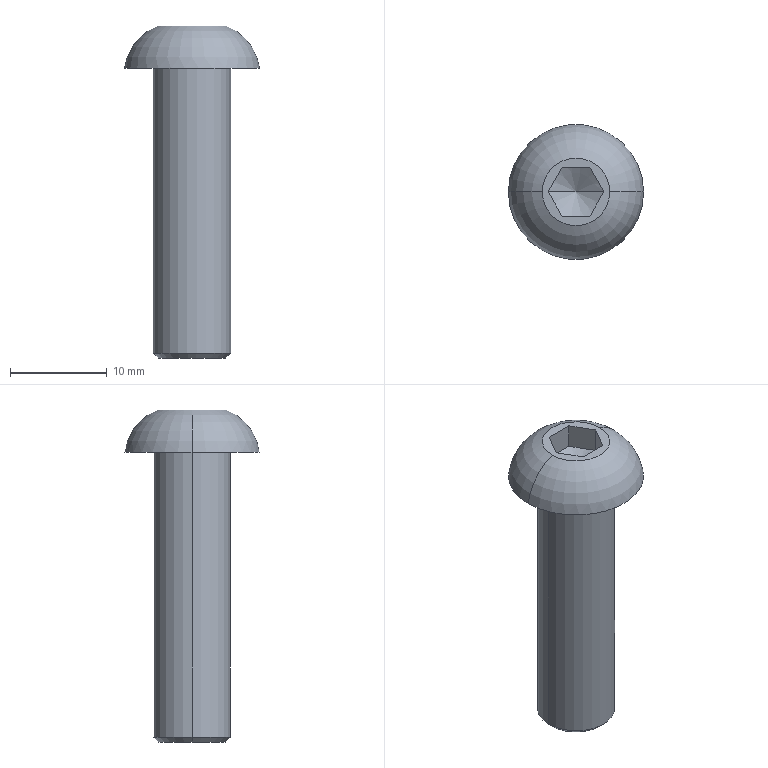Part | NX | features BREP 1 | 1 solid | 18 faces | box 14 x 14 x 34.4 mm | volume 1931 mm3 | plane 10 | cone 4 | torus 2 | cylinder 2 | commonest cylinder face diameters 8 x2
STEP:
#1=CARTESIAN_POINT('',(0.,0.,0.06795));
#2=VERTEX_POINT('',#1);
#3=CARTESIAN_POINT('',(-3.,0.,1.8));
#4=VERTEX_POINT('',#3);
#5=CARTESIAN_POINT('',(-3.,0.,1.8));
#6=DIRECTION('',(-0.866,0.,0.5));
#7=VECTOR('',#6,1000.);
#8=LINE('',#5,#7);
#9=EDGE_CURVE('',#2,#4,#8,.T.);
#10=ORIENTED_EDGE('',*,*,#9,.F.);
#11=CARTESIAN_POINT('',(3.,0.,1.8));
#12=VERTEX_POINT('',#11);
#13=CARTESIAN_POINT('',(3.,0.,1.8));
#14=DIRECTION('',(0.866,0.,0.5));
#15=VECTOR('',#14,1000.);
#16=LINE('',#13,#15);
#17=EDGE_CURVE('',#2,#12,#16,.T.);
#18=ORIENTED_EDGE('',*,*,#17,.T.);
#19=CARTESIAN_POINT('',(0.,0.,1.8));
#20=DIRECTION('',(0.,0.,-1.));
#21=DIRECTION('',(-1.,0.,0.));
#22=AXIS2_PLACEMENT_3D('',#19,#20,#21);
#23=CIRCLE('',#22,3.);
#24=EDGE_CURVE('',#4,#12,#23,.T.);
#25=ORIENTED_EDGE('',*,*,#24,.F.);
#26=EDGE_LOOP('',(#10,#18,#25));
#27=FACE_BOUND('',#26,.T.);
#28=CARTESIAN_POINT('',(0.,0.,1.8));
#29=DIRECTION('',(0.,0.,1.));
#30=DIRECTION('',(-1.,0.,0.));
#31=AXIS2_PLACEMENT_3D('',#28,#29,#30);
#32=CONICAL_SURFACE('',#31,3.,1.047);
#33=ADVANCED_FACE('',(#27),#32,.F.);
#34=CARTESIAN_POINT('',(-3.5,0.,-30.));
#35=VERTEX_POINT('',#34);
#36=CARTESIAN_POINT('',(3.5,0.,-30.));
#37=VERTEX_POINT('',#36);
#38=CARTESIAN_POINT('',(0.,0.,-30.));
#39=DIRECTION('',(0.,0.,1.));
#40=DIRECTION('',(-1.,0.,0.));
#41=AXIS2_PLACEMENT_3D('',#38,#39,#40);
#42=CIRCLE('',#41,3.5);
#43=EDGE_CURVE('',#35,#37,#42,.T.);
#44=ORIENTED_EDGE('',*,*,#43,.T.);
#45=CARTESIAN_POINT('',(4.,0.,-29.5));
#46=VERTEX_POINT('',#45);
#47=CARTESIAN_POINT('',(4.,0.,-29.5));
#48=DIRECTION('',(0.7071,0.,0.7071));
#49=VECTOR('',#48,1000.);
#50=LINE('',#47,#49);
#51=EDGE_CURVE('',#37,#46,#50,.T.);
#52=ORIENTED_EDGE('',*,*,#51,.T.);
#53=CARTESIAN_POINT('',(-4.,0.,-29.5));
#54=VERTEX_POINT('',#53);
#55=CARTESIAN_POINT('',(0.,0.,-29.5));
#56=DIRECTION('',(0.,0.,-1.));
#57=DIRECTION('',(-1.,0.,0.));
#58=AXIS2_PLACEMENT_3D('',#55,#56,#57);
#59=CIRCLE('',#58,4.);
#60=EDGE_CURVE('',#46,#54,#59,.T.);
#61=ORIENTED_EDGE('',*,*,#60,.T.);
#62=CARTESIAN_POINT('',(-4.,0.,-29.5));
#63=DIRECTION('',(-0.7071,0.,0.7071));
#64=VECTOR('',#63,1000.);
#65=LINE('',#62,#64);
#66=EDGE_CURVE('',#35,#54,#65,.T.);
#67=ORIENTED_EDGE('',*,*,#66,.F.);
#68=EDGE_LOOP('',(#44,#52,#61,#67));
#69=FACE_BOUND('',#68,.T.);
#70=CARTESIAN_POINT('',(0.,0.,-29.5));
#71=DIRECTION('',(0.,0.,1.));
#72=DIRECTION('',(-1.,0.,0.));
#73=AXIS2_PLACEMENT_3D('',#70,#71,#72);
#74=CONICAL_SURFACE('',#73,4.,0.7854);
#75=ADVANCED_FACE('',(#69),#74,.T.);
#76=CARTESIAN_POINT('',(7.,0.,0.));
#77=VERTEX_POINT('',#76);
#78=CARTESIAN_POINT('',(-7.,0.,0.));
#79=VERTEX_POINT('',#78);
#80=CARTESIAN_POINT('',(0.,0.,0.));
#81=DIRECTION('',(0.,0.,-1.));
#82=DIRECTION('',(-1.,0.,0.));
#83=AXIS2_PLACEMENT_3D('',#80,#81,#82);
#84=CIRCLE('',#83,7.);
#85=EDGE_CURVE('',#77,#79,#84,.T.);
#86=ORIENTED_EDGE('',*,*,#85,.F.);
#87=CARTESIAN_POINT('',(3.5,0.,4.4));
#88=VERTEX_POINT('',#87);
#89=CARTESIAN_POINT('',(1.642,0.,-0.6702));
#90=DIRECTION('',(0.,-1.,0.));
#91=DIRECTION('',(1.,0.,0.));
#92=AXIS2_PLACEMENT_3D('',#89,#90,#91);
#93=CIRCLE('',#92,5.4);
#94=EDGE_CURVE('',#77,#88,#93,.T.);
#95=ORIENTED_EDGE('',*,*,#94,.T.);
#96=CARTESIAN_POINT('',(-3.5,0.,4.4));
#97=VERTEX_POINT('',#96);
#98=CARTESIAN_POINT('',(0.,0.,4.4));
#99=DIRECTION('',(0.,0.,-1.));
#100=DIRECTION('',(-1.,0.,0.));
#101=AXIS2_PLACEMENT_3D('',#98,#99,#100);
#102=CIRCLE('',#101,3.5);
#103=EDGE_CURVE('',#88,#97,#102,.T.);
#104=ORIENTED_EDGE('',*,*,#103,.T.);
#105=CARTESIAN_POINT('',(-1.642,0.,-0.6702));
#106=DIRECTION('',(0.,1.,0.));
#107=DIRECTION('',(0.,0.,1.));
#108=AXIS2_PLACEMENT_3D('',#105,#106,#107);
#109=CIRCLE('',#108,5.4);
#110=EDGE_CURVE('',#79,#97,#109,.T.);
#111=ORIENTED_EDGE('',*,*,#110,.F.);
#112=EDGE_LOOP('',(#86,#95,#104,#111));
#113=FACE_BOUND('',#112,.T.);
#114=CARTESIAN_POINT('',(0.,0.,-0.6702));
#115=DIRECTION('',(0.,0.,1.));
#116=DIRECTION('',(-1.,0.,0.));
#117=AXIS2_PLACEMENT_3D('',#114,#115,#116);
#118=DEGENERATE_TOROIDAL_SURFACE('',#117,1.642,5.4,.T.);
#119=ADVANCED_FACE('',(#113),#118,.T.);
#120=ORIENTED_EDGE('',*,*,#60,.F.);
#121=CARTESIAN_POINT('',(4.,0.,0.));
#122=VERTEX_POINT('',#121);
#123=CARTESIAN_POINT('',(4.,0.,-30.));
#124=DIRECTION('',(0.,0.,1.));
#125=VECTOR('',#124,1000.);
#126=LINE('',#123,#125);
#127=EDGE_CURVE('',#46,#122,#126,.T.);
#128=ORIENTED_EDGE('',*,*,#127,.T.);
#129=CARTESIAN_POINT('',(-4.,0.,0.));
#130=VERTEX_POINT('',#129);
#131=CARTESIAN_POINT('',(0.,0.,0.));
#132=DIRECTION('',(0.,0.,1.));
#133=DIRECTION('',(1.,0.,0.));
#134=AXIS2_PLACEMENT_3D('',#131,#132,#133);
#135=CIRCLE('',#134,4.);
#136=EDGE_CURVE('',#130,#122,#135,.T.);
#137=ORIENTED_EDGE('',*,*,#136,.F.);
#138=CARTESIAN_POINT('',(-4.,0.,-30.));
#139=DIRECTION('',(0.,0.,1.));
#140=VECTOR('',#139,1000.);
#141=LINE('',#138,#140);
#142=EDGE_CURVE('',#54,#130,#141,.T.);
#143=ORIENTED_EDGE('',*,*,#142,.F.);
#144=EDGE_LOOP('',(#120,#128,#137,#143));
#145=FACE_BOUND('',#144,.T.);
#146=CARTESIAN_POINT('',(0.,0.,-30.));
#147=DIRECTION('',(0.,0.,1.));
#148=DIRECTION('',(-1.,0.,0.));
#149=AXIS2_PLACEMENT_3D('',#146,#147,#148);
#150=CYLINDRICAL_SURFACE('',#149,4.);
#151=ADVANCED_FACE('',(#145),#150,.T.);
#152=CARTESIAN_POINT('',(0.,0.,4.4));
#153=DIRECTION('',(0.,0.,-1.));
#154=DIRECTION('',(-1.,0.,0.));
#155=AXIS2_PLACEMENT_3D('',#152,#153,#154);
#156=CIRCLE('',#155,3.5);
#157=EDGE_CURVE('',#97,#88,#156,.T.);
#158=ORIENTED_EDGE('',*,*,#157,.F.);
#159=ORIENTED_EDGE('',*,*,#103,.F.);
#160=EDGE_LOOP('',(#158,#159));
#161=FACE_BOUND('',#160,.T.);
#162=CARTESIAN_POINT('',(2.887,0.,4.4));
#163=VERTEX_POINT('',#162);
#164=CARTESIAN_POINT('',(1.443,2.5,4.4));
#165=VERTEX_POINT('',#164);
#166=CARTESIAN_POINT('',(2.887,0.,4.4));
#167=DIRECTION('',(-0.5,0.866,0.));
#168=VECTOR('',#167,1000.);
#169=LINE('',#166,#168);
#170=EDGE_CURVE('',#163,#165,#169,.T.);
#171=ORIENTED_EDGE('',*,*,#170,.F.);
#172=CARTESIAN_POINT('',(1.443,-2.5,4.4));
#173=VERTEX_POINT('',#172);
#174=CARTESIAN_POINT('',(1.443,-2.5,4.4));
#175=DIRECTION('',(0.5,0.866,0.));
#176=VECTOR('',#175,1000.);
#177=LINE('',#174,#176);
#178=EDGE_CURVE('',#173,#163,#177,.T.);
#179=ORIENTED_EDGE('',*,*,#178,.F.);
#180=CARTESIAN_POINT('',(-1.443,-2.5,4.4));
#181=VERTEX_POINT('',#180);
#182=CARTESIAN_POINT('',(-1.443,-2.5,4.4));
#183=DIRECTION('',(1.,0.,0.));
#184=VECTOR('',#183,1000.);
#185=LINE('',#182,#184);
#186=EDGE_CURVE('',#181,#173,#185,.T.);
#187=ORIENTED_EDGE('',*,*,#186,.F.);
#188=CARTESIAN_POINT('',(-2.887,0.,4.4));
#189=VERTEX_POINT('',#188);
#190=CARTESIAN_POINT('',(-2.887,0.,4.4));
#191=DIRECTION('',(0.5,-0.866,0.));
#192=VECTOR('',#191,1000.);
#193=LINE('',#190,#192);
#194=EDGE_CURVE('',#189,#181,#193,.T.);
#195=ORIENTED_EDGE('',*,*,#194,.F.);
#196=CARTESIAN_POINT('',(-1.443,2.5,4.4));
#197=VERTEX_POINT('',#196);
#198=CARTESIAN_POINT('',(-1.443,2.5,4.4));
#199=DIRECTION('',(-0.5,-0.866,0.));
#200=VECTOR('',#199,1000.);
#201=LINE('',#198,#200);
#202=EDGE_CURVE('',#197,#189,#201,.T.);
#203=ORIENTED_EDGE('',*,*,#202,.F.);
#204=CARTESIAN_POINT('',(1.443,2.5,4.4));
#205=DIRECTION('',(-1.,0.,0.));
#206=VECTOR('',#205,1000.);
#207=LINE('',#204,#206);
#208=EDGE_CURVE('',#165,#197,#207,.T.);
#209=ORIENTED_EDGE('',*,*,#208,.F.);
#210=EDGE_LOOP('',(#171,#179,#187,#195,#203,#209));
#211=FACE_BOUND('',#210,.T.);
#212=CARTESIAN_POINT('',(0.,0.,4.4));
#213=DIRECTION('',(0.,0.,-1.));
#214=DIRECTION('',(0.,-1.,0.));
#215=AXIS2_PLACEMENT_3D('',#212,#213,#214);
#216=PLANE('',#215);
#217=ADVANCED_FACE('',(#161,#211),#216,.F.);
#218=CARTESIAN_POINT('',(0.,0.,0.));
#219=DIRECTION('',(0.,0.,-1.));
#220=DIRECTION('',(-1.,0.,0.));
#221=AXIS2_PLACEMENT_3D('',#218,#219,#220);
#222=CIRCLE('',#221,7.);
#223=EDGE_CURVE('',#79,#77,#222,.T.);
#224=ORIENTED_EDGE('',*,*,#223,.T.);
#225=ORIENTED_EDGE('',*,*,#85,.T.);
#226=EDGE_LOOP('',(#224,#225));
#227=FACE_BOUND('',#226,.T.);
#228=ORIENTED_EDGE('',*,*,#136,.T.);
#229=CARTESIAN_POINT('',(0.,0.,0.));
#230=DIRECTION('',(0.,0.,1.));
#231=DIRECTION('',(1.,0.,0.));
#232=AXIS2_PLACEMENT_3D('',#229,#230,#231);
#233=CIRCLE('',#232,4.);
#234=EDGE_CURVE('',#122,#130,#233,.T.);
#235=ORIENTED_EDGE('',*,*,#234,.T.);
#236=EDGE_LOOP('',(#228,#235));
#237=FACE_BOUND('',#236,.T.);
#238=CARTESIAN_POINT('',(0.,0.,0.));
#239=DIRECTION('',(0.,0.,-1.));
#240=DIRECTION('',(0.,-1.,0.));
#241=AXIS2_PLACEMENT_3D('',#238,#239,#240);
#242=PLANE('',#241);
#243=ADVANCED_FACE('',(#227,#237),#242,.T.);
#244=ORIENTED_EDGE('',*,*,#127,.F.);
#245=CARTESIAN_POINT('',(0.,0.,-29.5));
#246=DIRECTION('',(0.,0.,-1.));
#247=DIRECTION('',(-1.,0.,0.));
#248=AXIS2_PLACEMENT_3D('',#245,#246,#247);
#249=CIRCLE('',#248,4.);
#250=EDGE_CURVE('',#54,#46,#249,.T.);
#251=ORIENTED_EDGE('',*,*,#250,.F.);
#252=ORIENTED_EDGE('',*,*,#142,.T.);
#253=ORIENTED_EDGE('',*,*,#234,.F.);
#254=EDGE_LOOP('',(#244,#251,#252,#253));
#255=FACE_BOUND('',#254,.T.);
#256=CARTESIAN_POINT('',(0.,0.,-30.));
#257=DIRECTION('',(0.,0.,1.));
#258=DIRECTION('',(-1.,0.,0.));
#259=AXIS2_PLACEMENT_3D('',#256,#257,#258);
#260=CYLINDRICAL_SURFACE('',#259,4.);
#261=ADVANCED_FACE('',(#255),#260,.T.);
#262=ORIENTED_EDGE('',*,*,#43,.F.);
#263=CARTESIAN_POINT('',(0.,0.,-30.));
#264=DIRECTION('',(0.,0.,1.));
#265=DIRECTION('',(-1.,0.,0.));
#266=AXIS2_PLACEMENT_3D('',#263,#264,#265);
#267=CIRCLE('',#266,3.5);
#268=EDGE_CURVE('',#37,#35,#267,.T.);
#269=ORIENTED_EDGE('',*,*,#268,.F.);
#270=EDGE_LOOP('',(#262,#269));
#271=FACE_BOUND('',#270,.T.);
#272=CARTESIAN_POINT('',(0.,0.,-30.));
#273=DIRECTION('',(0.,0.,1.));
#274=DIRECTION('',(1.,0.,0.));
#275=AXIS2_PLACEMENT_3D('',#272,#273,#274);
#276=PLANE('',#275);
#277=ADVANCED_FACE('',(#271),#276,.F.);
#278=ORIENTED_EDGE('',*,*,#94,.F.);
#279=ORIENTED_EDGE('',*,*,#223,.F.);
#280=ORIENTED_EDGE('',*,*,#110,.T.);
#281=ORIENTED_EDGE('',*,*,#157,.T.);
#282=EDGE_LOOP('',(#278,#279,#280,#281));
#283=FACE_BOUND('',#282,.T.);
#284=CARTESIAN_POINT('',(0.,0.,-0.6702));
#285=DIRECTION('',(0.,0.,1.));
#286=DIRECTION('',(-1.,0.,0.));
#287=AXIS2_PLACEMENT_3D('',#284,#285,#286);
#288=DEGENERATE_TOROIDAL_SURFACE('',#287,1.642,5.4,.T.);
#289=ADVANCED_FACE('',(#283),#288,.T.);
#290=ORIENTED_EDGE('',*,*,#51,.F.);
#291=ORIENTED_EDGE('',*,*,#268,.T.);
#292=ORIENTED_EDGE('',*,*,#66,.T.);
#293=ORIENTED_EDGE('',*,*,#250,.T.);
#294=EDGE_LOOP('',(#290,#291,#292,#293));
#295=FACE_BOUND('',#294,.T.);
#296=CARTESIAN_POINT('',(0.,0.,-29.5));
#297=DIRECTION('',(0.,0.,1.));
#298=DIRECTION('',(-1.,0.,0.));
#299=AXIS2_PLACEMENT_3D('',#296,#297,#298);
#300=CONICAL_SURFACE('',#299,4.,0.7854);
#301=ADVANCED_FACE('',(#295),#300,.T.);
#302=ORIENTED_EDGE('',*,*,#170,.T.);
#303=CARTESIAN_POINT('',(1.443,2.5,1.8));
#304=VERTEX_POINT('',#303);
#305=CARTESIAN_POINT('',(1.443,2.5,1.8));
#306=DIRECTION('',(0.,0.,1.));
#307=VECTOR('',#306,1000.);
#308=LINE('',#305,#307);
#309=EDGE_CURVE('',#304,#165,#308,.T.);
#310=ORIENTED_EDGE('',*,*,#309,.F.);
#311=CARTESIAN_POINT('',(2.887,0.,1.8));
#312=VERTEX_POINT('',#311);
#313=CARTESIAN_POINT('',(2.887,0.,1.8));
#314=DIRECTION('',(-0.5,0.866,0.));
#315=VECTOR('',#314,1000.);
#316=LINE('',#313,#315);
#317=EDGE_CURVE('',#312,#304,#316,.T.);
#318=ORIENTED_EDGE('',*,*,#317,.F.);
#319=CARTESIAN_POINT('',(2.887,0.,1.8));
#320=DIRECTION('',(0.,0.,1.));
#321=VECTOR('',#320,1000.);
#322=LINE('',#319,#321);
#323=EDGE_CURVE('',#312,#163,#322,.T.);
#324=ORIENTED_EDGE('',*,*,#323,.T.);
#325=EDGE_LOOP('',(#302,#310,#318,#324));
#326=FACE_BOUND('',#325,.T.);
#327=CARTESIAN_POINT('',(2.887,0.,1.8));
#328=DIRECTION('',(-0.866,-0.5,0.));
#329=DIRECTION('',(-0.5,0.866,0.));
#330=AXIS2_PLACEMENT_3D('',#327,#328,#329);
#331=PLANE('',#330);
#332=ADVANCED_FACE('',(#326),#331,.T.);
#333=ORIENTED_EDGE('',*,*,#208,.T.);
#334=CARTESIAN_POINT('',(-1.443,2.5,1.8));
#335=VERTEX_POINT('',#334);
#336=CARTESIAN_POINT('',(-1.443,2.5,1.8));
#337=DIRECTION('',(0.,0.,1.));
#338=VECTOR('',#337,1000.);
#339=LINE('',#336,#338);
#340=EDGE_CURVE('',#335,#197,#339,.T.);
#341=ORIENTED_EDGE('',*,*,#340,.F.);
#342=CARTESIAN_POINT('',(1.443,2.5,1.8));
#343=DIRECTION('',(-1.,0.,0.));
#344=VECTOR('',#343,1000.);
#345=LINE('',#342,#344);
#346=EDGE_CURVE('',#304,#335,#345,.T.);
#347=ORIENTED_EDGE('',*,*,#346,.F.);
#348=ORIENTED_EDGE('',*,*,#309,.T.);
#349=EDGE_LOOP('',(#333,#341,#347,#348));
#350=FACE_BOUND('',#349,.T.);
#351=CARTESIAN_POINT('',(1.443,2.5,1.8));
#352=DIRECTION('',(0.,-1.,0.));
#353=DIRECTION('',(0.,0.,-1.));
#354=AXIS2_PLACEMENT_3D('',#351,#352,#353);
#355=PLANE('',#354);
#356=ADVANCED_FACE('',(#350),#355,.T.);
#357=ORIENTED_EDGE('',*,*,#202,.T.);
#358=CARTESIAN_POINT('',(-2.887,0.,1.8));
#359=VERTEX_POINT('',#358);
#360=CARTESIAN_POINT('',(-2.887,0.,1.8));
#361=DIRECTION('',(0.,0.,1.));
#362=VECTOR('',#361,1000.);
#363=LINE('',#360,#362);
#364=EDGE_CURVE('',#359,#189,#363,.T.);
#365=ORIENTED_EDGE('',*,*,#364,.F.);
#366=CARTESIAN_POINT('',(-1.443,2.5,1.8));
#367=DIRECTION('',(-0.5,-0.866,0.));
#368=VECTOR('',#367,1000.);
#369=LINE('',#366,#368);
#370=EDGE_CURVE('',#335,#359,#369,.T.);
#371=ORIENTED_EDGE('',*,*,#370,.F.);
#372=ORIENTED_EDGE('',*,*,#340,.T.);
#373=EDGE_LOOP('',(#357,#365,#371,#372));
#374=FACE_BOUND('',#373,.T.);
#375=CARTESIAN_POINT('',(-1.443,2.5,1.8));
#376=DIRECTION('',(0.866,-0.5,0.));
#377=DIRECTION('',(0.,0.,-1.));
#378=AXIS2_PLACEMENT_3D('',#375,#376,#377);
#379=PLANE('',#378);
#380=ADVANCED_FACE('',(#374),#379,.T.);
#381=ORIENTED_EDGE('',*,*,#194,.T.);
#382=CARTESIAN_POINT('',(-1.443,-2.5,1.8));
#383=VERTEX_POINT('',#382);
#384=CARTESIAN_POINT('',(-1.443,-2.5,1.8));
#385=DIRECTION('',(0.,0.,1.));
#386=VECTOR('',#385,1000.);
#387=LINE('',#384,#386);
#388=EDGE_CURVE('',#383,#181,#387,.T.);
#389=ORIENTED_EDGE('',*,*,#388,.F.);
#390=CARTESIAN_POINT('',(-2.887,0.,1.8));
#391=DIRECTION('',(0.5,-0.866,0.));
#392=VECTOR('',#391,1000.);
#393=LINE('',#390,#392);
#394=EDGE_CURVE('',#359,#383,#393,.T.);
#395=ORIENTED_EDGE('',*,*,#394,.F.);
#396=ORIENTED_EDGE('',*,*,#364,.T.);
#397=EDGE_LOOP('',(#381,#389,#395,#396));
#398=FACE_BOUND('',#397,.T.);
#399=CARTESIAN_POINT('',(-2.887,0.,1.8));
#400=DIRECTION('',(0.866,0.5,0.));
#401=DIRECTION('',(0.,0.,-1.));
#402=AXIS2_PLACEMENT_3D('',#399,#400,#401);
#403=PLANE('',#402);
#404=ADVANCED_FACE('',(#398),#403,.T.);
#405=ORIENTED_EDGE('',*,*,#186,.T.);
#406=CARTESIAN_POINT('',(1.443,-2.5,1.8));
#407=VERTEX_POINT('',#406);
#408=CARTESIAN_POINT('',(1.443,-2.5,1.8));
#409=DIRECTION('',(0.,0.,1.));
#410=VECTOR('',#409,1000.);
#411=LINE('',#408,#410);
#412=EDGE_CURVE('',#407,#173,#411,.T.);
#413=ORIENTED_EDGE('',*,*,#412,.F.);
#414=CARTESIAN_POINT('',(-1.443,-2.5,1.8));
#415=DIRECTION('',(1.,0.,0.));
#416=VECTOR('',#415,1000.);
#417=LINE('',#414,#416);
#418=EDGE_CURVE('',#383,#407,#417,.T.);
#419=ORIENTED_EDGE('',*,*,#418,.F.);
#420=ORIENTED_EDGE('',*,*,#388,.T.);
#421=EDGE_LOOP('',(#405,#413,#419,#420));
#422=FACE_BOUND('',#421,.T.);
#423=CARTESIAN_POINT('',(-1.443,-2.5,1.8));
#424=DIRECTION('',(0.,1.,0.));
#425=DIRECTION('',(1.,0.,0.));
#426=AXIS2_PLACEMENT_3D('',#423,#424,#425);
#427=PLANE('',#426);
#428=ADVANCED_FACE('',(#422),#427,.T.);
#429=ORIENTED_EDGE('',*,*,#178,.T.);
#430=ORIENTED_EDGE('',*,*,#323,.F.);
#431=CARTESIAN_POINT('',(1.443,-2.5,1.8));
#432=DIRECTION('',(0.5,0.866,0.));
#433=VECTOR('',#432,1000.);
#434=LINE('',#431,#433);
#435=EDGE_CURVE('',#407,#312,#434,.T.);
#436=ORIENTED_EDGE('',*,*,#435,.F.);
#437=ORIENTED_EDGE('',*,*,#412,.T.);
#438=EDGE_LOOP('',(#429,#430,#436,#437));
#439=FACE_BOUND('',#438,.T.);
#440=CARTESIAN_POINT('',(1.443,-2.5,1.8));
#441=DIRECTION('',(-0.866,0.5,0.));
#442=DIRECTION('',(0.,0.,1.));
#443=AXIS2_PLACEMENT_3D('',#440,#441,#442);
#444=PLANE('',#443);
#445=ADVANCED_FACE('',(#439),#444,.T.);
#446=ORIENTED_EDGE('',*,*,#24,.T.);
#447=CARTESIAN_POINT('',(0.,0.,1.8));
#448=DIRECTION('',(0.,0.,-1.));
#449=DIRECTION('',(-1.,0.,0.));
#450=AXIS2_PLACEMENT_3D('',#447,#448,#449);
#451=CIRCLE('',#450,3.);
#452=EDGE_CURVE('',#12,#4,#451,.T.);
#453=ORIENTED_EDGE('',*,*,#452,.T.);
#454=EDGE_LOOP('',(#446,#453));
#455=FACE_BOUND('',#454,.T.);
#456=ORIENTED_EDGE('',*,*,#317,.T.);
#457=ORIENTED_EDGE('',*,*,#346,.T.);
#458=ORIENTED_EDGE('',*,*,#370,.T.);
#459=ORIENTED_EDGE('',*,*,#394,.T.);
#460=ORIENTED_EDGE('',*,*,#418,.T.);
#461=ORIENTED_EDGE('',*,*,#435,.T.);
#462=EDGE_LOOP('',(#456,#457,#458,#459,#460,#461));
#463=FACE_BOUND('',#462,.T.);
#464=CARTESIAN_POINT('',(-3.,0.,1.8));
#465=DIRECTION('',(0.,0.,1.));
#466=DIRECTION('',(1.,0.,0.));
#467=AXIS2_PLACEMENT_3D('',#464,#465,#466);
#468=PLANE('',#467);
#469=ADVANCED_FACE('',(#455,#463),#468,.F.);
#470=ORIENTED_EDGE('',*,*,#17,.F.);
#471=ORIENTED_EDGE('',*,*,#9,.T.);
#472=ORIENTED_EDGE('',*,*,#452,.F.);
#473=EDGE_LOOP('',(#470,#471,#472));
#474=FACE_BOUND('',#473,.T.);
#475=CARTESIAN_POINT('',(0.,0.,1.8));
#476=DIRECTION('',(0.,0.,1.));
#477=DIRECTION('',(-1.,0.,0.));
#478=AXIS2_PLACEMENT_3D('',#475,#476,#477);
#479=CONICAL_SURFACE('',#478,3.,1.047);
#480=ADVANCED_FACE('',(#474),#479,.F.);
#481=CLOSED_SHELL('',(#33,#75,#119,#151,#217,#243,#261,#277,#289,#301,#332,#356,#380,#404,#428,#445,#469,#480));
#482=MANIFOLD_SOLID_BREP('',#481);
#483=(LENGTH_UNIT()NAMED_UNIT(*)SI_UNIT(.MILLI.,.METRE.));
#484=UNCERTAINTY_MEASURE_WITH_UNIT(LENGTH_MEASURE(0.00001),#483,'','');
#485=(NAMED_UNIT(*)PLANE_ANGLE_UNIT()SI_UNIT($,.RADIAN.));
#486=(NAMED_UNIT(*)SI_UNIT($,.STERADIAN.)SOLID_ANGLE_UNIT());
#487=(GEOMETRIC_REPRESENTATION_CONTEXT(3)GLOBAL_UNCERTAINTY_ASSIGNED_CONTEXT((#484))GLOBAL_UNIT_ASSIGNED_CONTEXT((#483,#485,#486))REPRESENTATION_CONTEXT('',''));
#488=ADVANCED_BREP_SHAPE_REPRESENTATION('',(#482),#487);